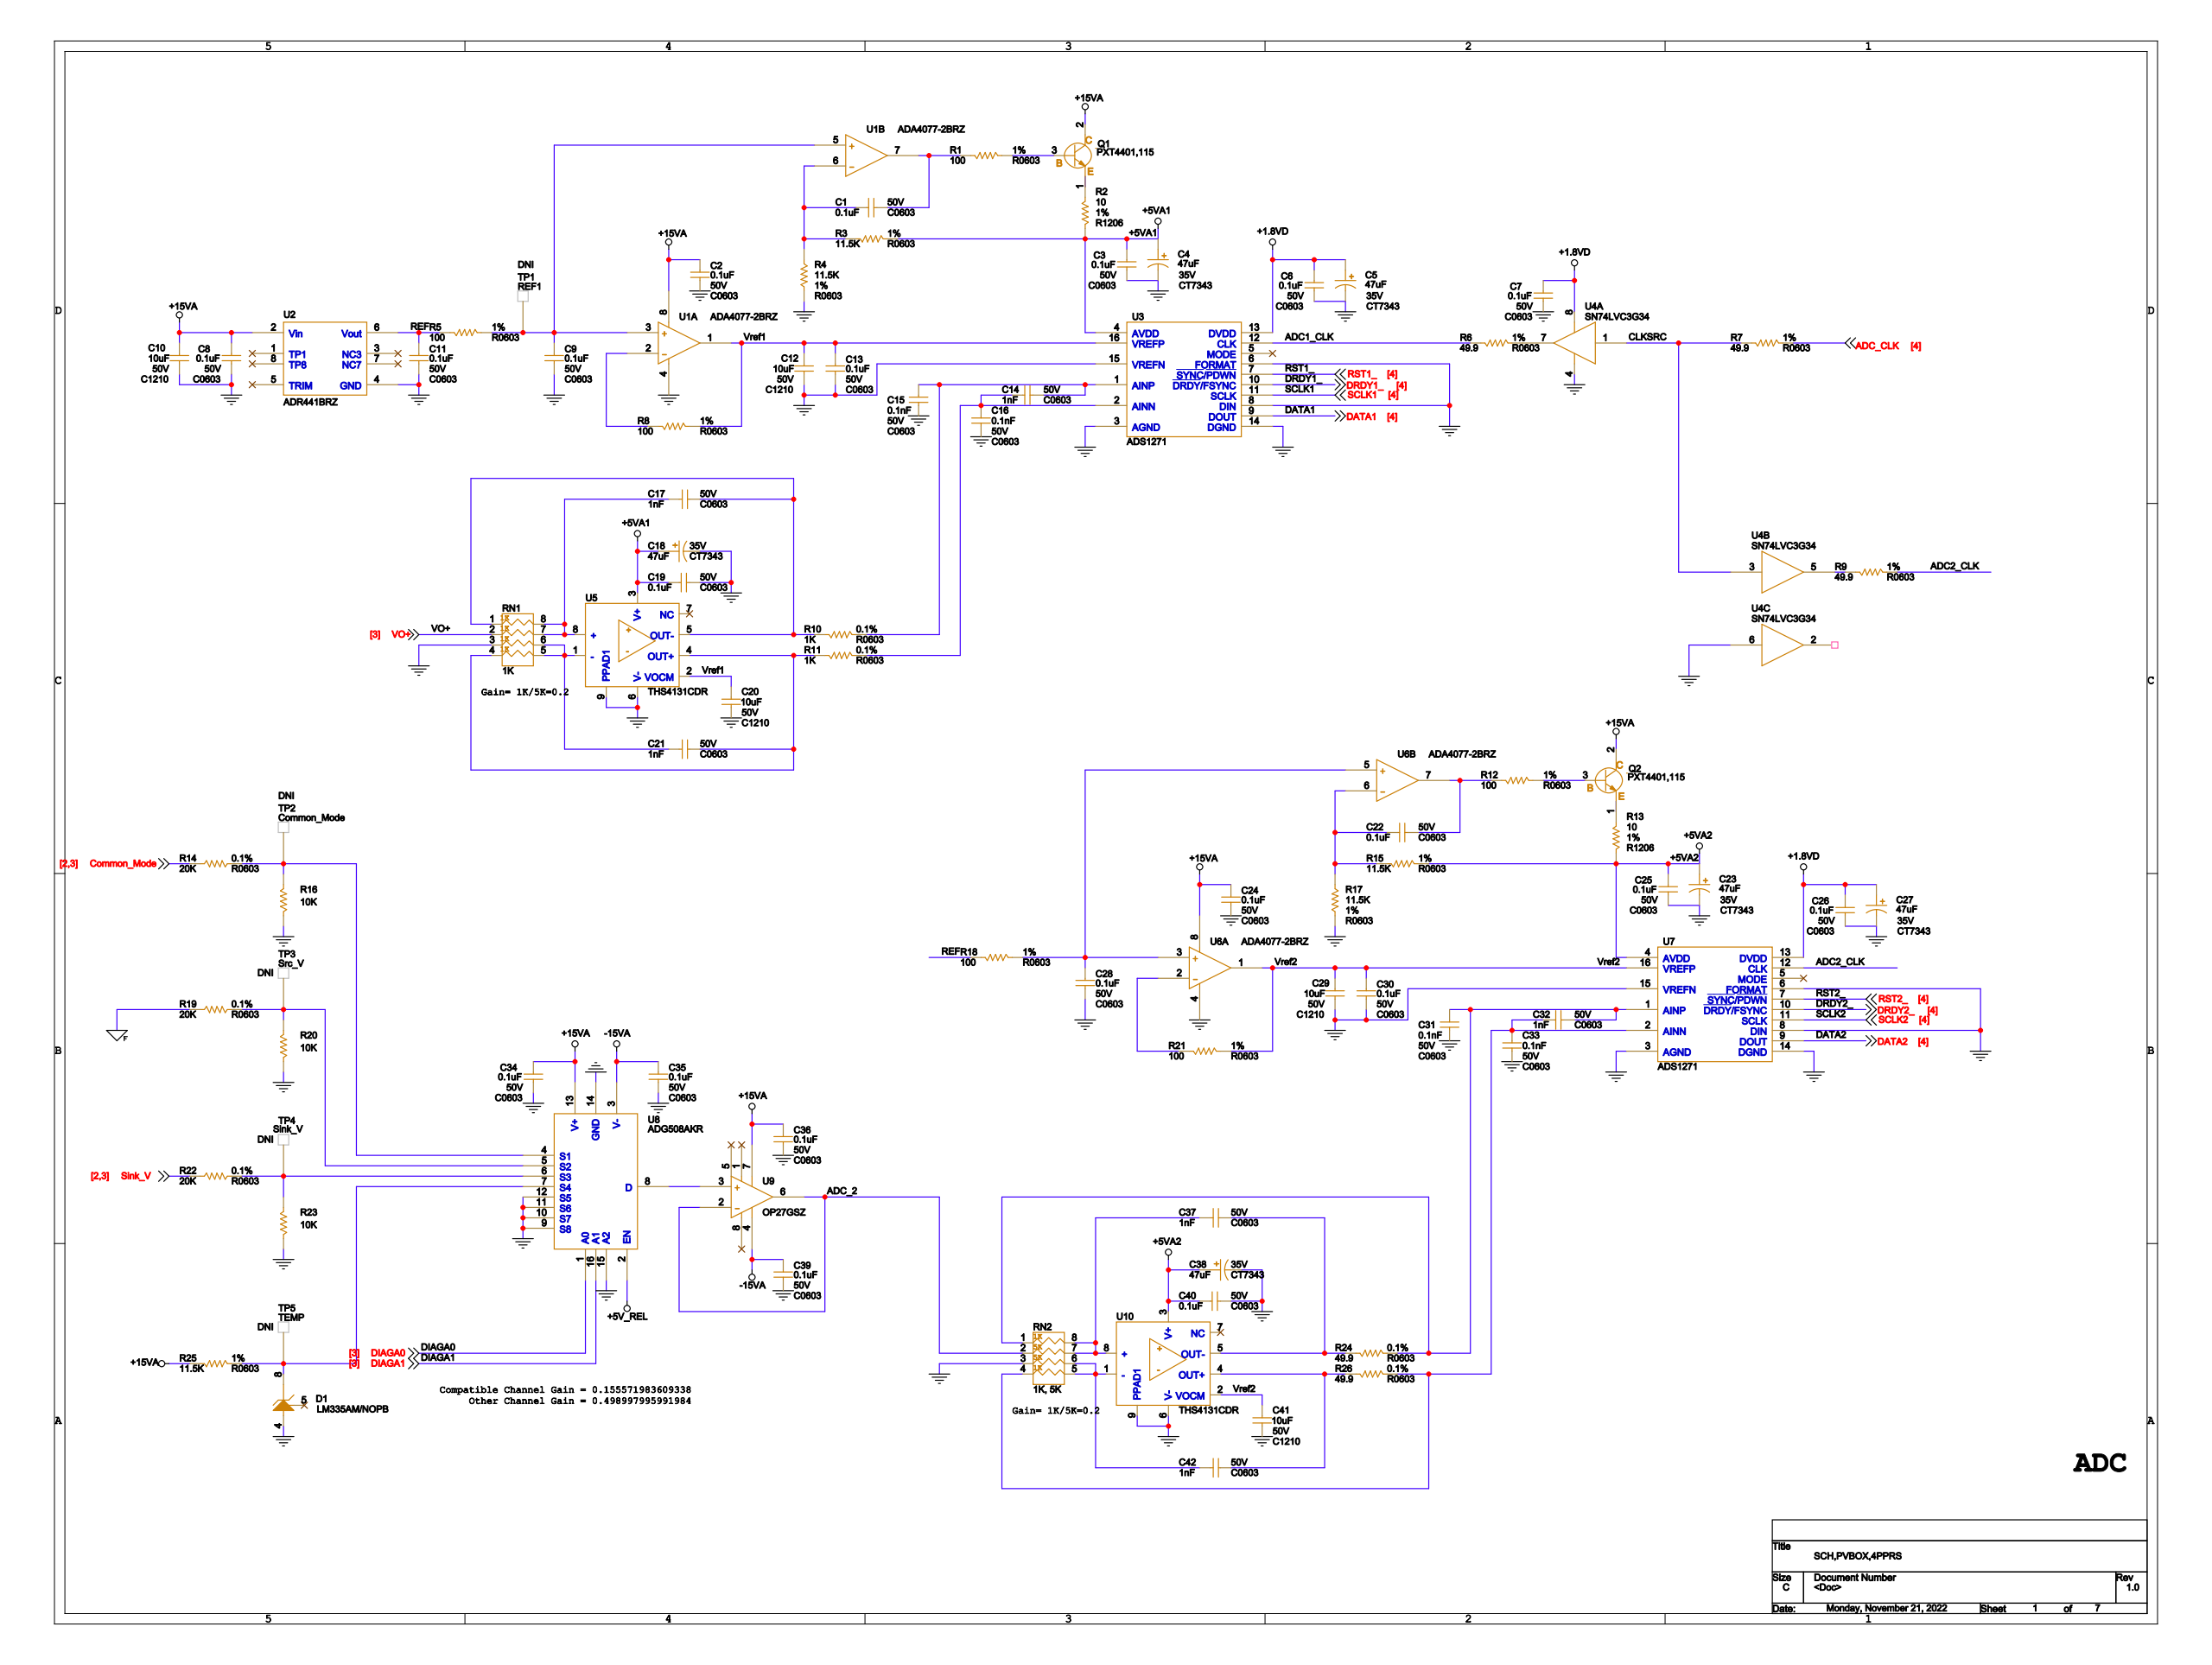Circuit board | Cadence Allegro | 405 parts | 254 nets | one sheet of the schematic
Parts on this sheet (reference | value | footprint):
C2 | C0603
C3 | C0603
C4 | CT7343
C8 | C0603
C10 | C1210
C11 | C0603
C17 | C0603
C18 | CT7343
C19 | C0603
C20 | C1210
C21 | C0603
C22 | C0603
C23 | CT7343
C24 | C0603
C25 | C0603
C26 | C0603
C27 | CT7343
C28 | C0603
C29 | C1210
C30 | C0603
C31 | C0603
C32 | C0603
C33 | C0603
C34 | C0603
C35 | C0603
C36 | C0603
C37 | C0603
C38 | CT7343
C39 | C0603
C40 | C0603
C41 | C1210
C42 | C0603
Q1 | SOT_3_2M6X4M6X1M6_1M5_C
Q2 | SOT_3_2M6X4M6X1M6_1M5_C
R2 | R1206
R3 | R0603
R5 | R0603
R6 | R0603
R7 | R0603
R9 | R0603
R13 | R1206
R15 | R0603
R17 | R0603
R18 | R0603
R19 | R0603
R20 | R0603
R21 | R0603
R22 | R0603
R23 | R0603
R24 | R0603
R25 | R0603
R26 | R0603
RN1 | ACASA
RN2 | ACASA
TP2 | TP_0M8X1M15
TP3 | TP_0M8X1M15
TP4 | TP_0M8X1M15
TP5 | TP_0M8X1M15
U2 | SOIC_8_4MX5MX1M75_1M27
U3 | SOPTS_16_4M5X5M1X1M2_0M65
U5 | SOIC8
U7 | SOPTS_16_4M5X5M1X1M2_0M65
U8 | SOIC_16_4MX10MX1M75_1M27
U9 | SOIC_8_4MX5MX1M75_1M27
U10 | SOIC8
Nets of these parts (net: part-pin ...):
GND: C2-2 C3-2 C4-2 C8-2 C10-2 C11-2 C18-2 C19-2 C20-2 C23-2 C24-2 C25-2 C26-2 C27-2 C28-2 C29-2 C30-2 C31-2 C33-2 C34-2 C35-2 C36-2 C38-2 C39-2 C40-2 C41-2 R17-1 R20-1 R23-1 RN1-3 RN2-3 U2-4 U3-3 U3-6 U3-8 U3-14 U3-15 U5-6 U5-9 U7-3 U7-6 U7-8 U7-14 U7-15 U8-9 U8-10 U8-11 U8-12 U8-14 U8-15 U10-6 U10-9
N17859090: C37-1 R24-1 U10-5
N19313234: C31-1 C32-2 R24-2 RN2-1 U7-1
N17859088: C42-1 R26-1 U10-4
N19313242: C32-1 C33-1 R26-2 RN2-4 U7-2
ADC1_CLK: R6-1 U3-12
N193142601: R6-2
CLKSRC: R7-1
ADC_CLK: R7-2
N19313191: R9-1
ADC2_CLK: R9-2 U7-12
N16962547: R3-2
REF: C11-1 R5-1 R18-1 U2-6
+1.8VD: C26-1 C27-1 U3-13 U7-13
VREF1: C20-1 U3-16 U5-2
GNDF: R19-1
+5V_REL: U8-2
+5VA1: C3-1 C4-1 C18-1 C19-1 R2-2 R3-1 U3-4 U5-3
+15VA: C2-1 C8-1 C10-1 C24-1 C34-1 C36-1 Q1-2 Q2-2 R25-1 U2-2 U8-13 U9-7
N19759059: C22-1 R15-2 R17-2
N19759051: C22-2
+5VA2: C23-1 C25-1 C38-1 C40-1 R13-2 R15-1 U7-4 U10-3
N19759037: C28-1 R18-2
VREF2: C29-1 C30-1 C41-1 R21-2 U7-16 U10-2
-15VA: C35-1 C39-1 U8-3 U9-4
N16961896: R5-2
N19313183: U3-2
N19313186: U3-1
N18208446: C17-1 RN1-1 U5-5
N19313443: C17-2 RN1-7 RN1-8 U5-8
N18208464: C21-1 RN1-4 U5-4
N19313456: C21-2 RN1-5 RN1-6 U5-1
N19313490: C37-2 RN2-7 RN2-8 U10-8
N17859211: C42-2 RN2-5 RN2-6 U10-1
N19313530: R25-2 TP5-1 U8-7
SINK_V: R22-1
N19313228: Q1-3
N19313231: Q1-1 R2-1
N19759057: Q2-3
N19759063: Q2-1 R13-1
N19759187: R21-1
N18025238: TP2-1 U8-4
N18157893: R19-2 R20-2 TP3-1 U8-5
N18157647: R22-2 R23-2 TP4-1 U8-6
VO+: RN1-2
ADC_2: RN2-2 U9-2 U9-6
N19313356: U8-8 U9-3
DIAGA1: U8-16
DIAGA0: U8-1
DATA1: U3-9
DRDY1_: U3-10
SCLK1: U3-11
RST1_: U3-7
DATA2: U7-9
DRDY2_: U7-10
SCLK2: U7-11
RST2_: U7-7